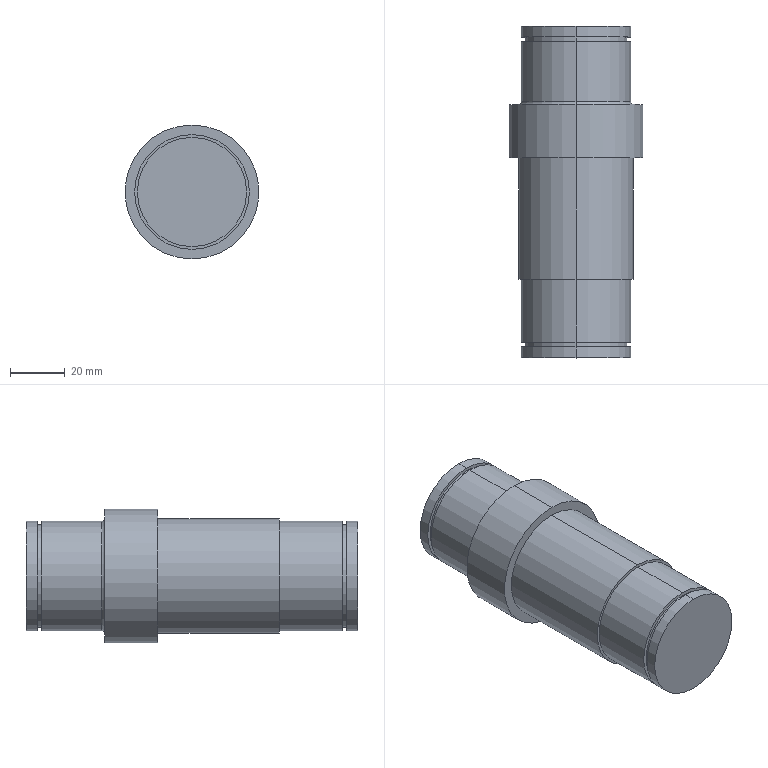Part | STEP file | 03-Pin shaft 1 | 1 solid | 27 faces | box 49 x 121.4 x 49 mm | volume 170065 mm3 | cylinder 16 | plane 9 | torus 2 | commonest cylinder face diameters 40 x8 37.5 x4 42 x2 49 x2